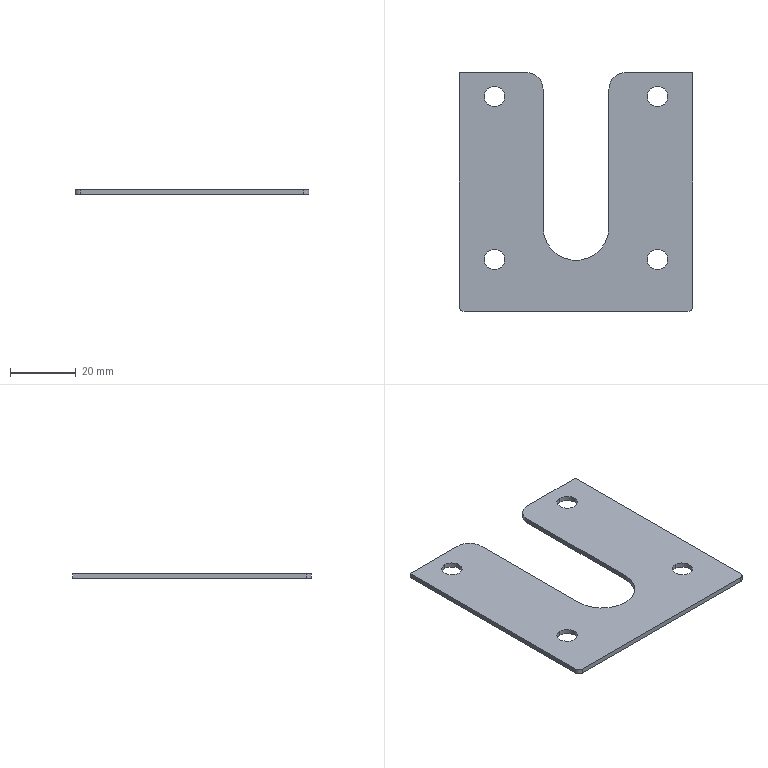Part | NX | features solid 2 | 1 solid | 22 faces | box 71 x 72.5 x 1.5 mm | volume 5877 mm3 | cylinder 13 | plane 9 | commonest cylinder face diameters 6.2 x8 3 x2 10 x2 20 x1
STEP:
#1=CARTESIAN_POINT('',(-1034.749,-1371.151,1295.));
#2=VERTEX_POINT('',#1);
#3=CARTESIAN_POINT('',(-1034.749,-1371.151,1296.5));
#4=VERTEX_POINT('',#3);
#5=CARTESIAN_POINT('',(-1034.749,-1371.151,1395.));
#6=DIRECTION('',(0.,0.,-1.));
#7=VECTOR('',#6,1000.);
#8=LINE('',#5,#7);
#9=EDGE_CURVE('',#2,#4,#8,.F.);
#10=ORIENTED_EDGE('',*,*,#9,.T.);
#11=CARTESIAN_POINT('',(-1034.749,-1377.351,1296.5));
#12=VERTEX_POINT('',#11);
#13=CARTESIAN_POINT('',(-1034.749,-1374.251,1296.5));
#14=DIRECTION('',(0.,0.,1.));
#15=DIRECTION('',(1.,0.,0.));
#16=AXIS2_PLACEMENT_3D('',#13,#14,#15);
#17=CIRCLE('',#16,3.1);
#18=EDGE_CURVE('',#4,#12,#17,.T.);
#19=ORIENTED_EDGE('',*,*,#18,.T.);
#20=CARTESIAN_POINT('',(-1034.749,-1377.351,1295.));
#21=VERTEX_POINT('',#20);
#22=CARTESIAN_POINT('',(-1034.749,-1377.351,1395.));
#23=DIRECTION('',(0.,0.,-1.));
#24=VECTOR('',#23,1000.);
#25=LINE('',#22,#24);
#26=EDGE_CURVE('',#12,#21,#25,.T.);
#27=ORIENTED_EDGE('',*,*,#26,.T.);
#28=CARTESIAN_POINT('',(-1034.749,-1374.251,1295.));
#29=DIRECTION('',(0.,0.,1.));
#30=DIRECTION('',(1.,0.,0.));
#31=AXIS2_PLACEMENT_3D('',#28,#29,#30);
#32=CIRCLE('',#31,3.1);
#33=EDGE_CURVE('',#2,#21,#32,.T.);
#34=ORIENTED_EDGE('',*,*,#33,.F.);
#35=EDGE_LOOP('',(#10,#19,#27,#34));
#36=FACE_BOUND('',#35,.T.);
#37=CARTESIAN_POINT('',(-1034.749,-1374.251,1395.));
#38=DIRECTION('',(0.,0.,-1.));
#39=DIRECTION('',(0.,-1.,0.));
#40=AXIS2_PLACEMENT_3D('',#37,#38,#39);
#41=CYLINDRICAL_SURFACE('',#40,3.1);
#42=ADVANCED_FACE('',(#36),#41,.F.);
#43=CARTESIAN_POINT('',(-1034.749,-1420.649,1296.5));
#44=VERTEX_POINT('',#43);
#45=CARTESIAN_POINT('',(-1034.749,-1420.649,1295.));
#46=VERTEX_POINT('',#45);
#47=CARTESIAN_POINT('',(-1034.749,-1420.649,1395.));
#48=DIRECTION('',(0.,0.,-1.));
#49=VECTOR('',#48,1000.);
#50=LINE('',#47,#49);
#51=EDGE_CURVE('',#44,#46,#50,.T.);
#52=ORIENTED_EDGE('',*,*,#51,.F.);
#53=CARTESIAN_POINT('',(-1034.749,-1426.849,1296.5));
#54=VERTEX_POINT('',#53);
#55=CARTESIAN_POINT('',(-1034.749,-1423.749,1296.5));
#56=DIRECTION('',(0.,0.,1.));
#57=DIRECTION('',(1.,0.,0.));
#58=AXIS2_PLACEMENT_3D('',#55,#56,#57);
#59=CIRCLE('',#58,3.1);
#60=EDGE_CURVE('',#44,#54,#59,.T.);
#61=ORIENTED_EDGE('',*,*,#60,.T.);
#62=CARTESIAN_POINT('',(-1034.749,-1426.849,1295.));
#63=VERTEX_POINT('',#62);
#64=CARTESIAN_POINT('',(-1034.749,-1426.849,1395.));
#65=DIRECTION('',(0.,0.,-1.));
#66=VECTOR('',#65,1000.);
#67=LINE('',#64,#66);
#68=EDGE_CURVE('',#63,#54,#67,.F.);
#69=ORIENTED_EDGE('',*,*,#68,.F.);
#70=CARTESIAN_POINT('',(-1034.749,-1423.749,1295.));
#71=DIRECTION('',(0.,0.,1.));
#72=DIRECTION('',(1.,0.,0.));
#73=AXIS2_PLACEMENT_3D('',#70,#71,#72);
#74=CIRCLE('',#73,3.1);
#75=EDGE_CURVE('',#46,#63,#74,.T.);
#76=ORIENTED_EDGE('',*,*,#75,.F.);
#77=EDGE_LOOP('',(#52,#61,#69,#76));
#78=FACE_BOUND('',#77,.T.);
#79=CARTESIAN_POINT('',(-1034.749,-1423.749,1395.));
#80=DIRECTION('',(0.,0.,-1.));
#81=DIRECTION('',(0.,-1.,0.));
#82=AXIS2_PLACEMENT_3D('',#79,#80,#81);
#83=CYLINDRICAL_SURFACE('',#82,3.1);
#84=ADVANCED_FACE('',(#78),#83,.F.);
#85=CARTESIAN_POINT('',(-985.251,-1420.649,1295.));
#86=VERTEX_POINT('',#85);
#87=CARTESIAN_POINT('',(-985.251,-1420.649,1296.5));
#88=VERTEX_POINT('',#87);
#89=CARTESIAN_POINT('',(-985.251,-1420.649,1395.));
#90=DIRECTION('',(0.,0.,-1.));
#91=VECTOR('',#90,1000.);
#92=LINE('',#89,#91);
#93=EDGE_CURVE('',#86,#88,#92,.F.);
#94=ORIENTED_EDGE('',*,*,#93,.T.);
#95=CARTESIAN_POINT('',(-985.251,-1426.849,1296.5));
#96=VERTEX_POINT('',#95);
#97=CARTESIAN_POINT('',(-985.251,-1423.749,1296.5));
#98=DIRECTION('',(0.,0.,1.));
#99=DIRECTION('',(1.,0.,0.));
#100=AXIS2_PLACEMENT_3D('',#97,#98,#99);
#101=CIRCLE('',#100,3.1);
#102=EDGE_CURVE('',#88,#96,#101,.T.);
#103=ORIENTED_EDGE('',*,*,#102,.T.);
#104=CARTESIAN_POINT('',(-985.251,-1426.849,1295.));
#105=VERTEX_POINT('',#104);
#106=CARTESIAN_POINT('',(-985.251,-1426.849,1395.));
#107=DIRECTION('',(0.,0.,-1.));
#108=VECTOR('',#107,1000.);
#109=LINE('',#106,#108);
#110=EDGE_CURVE('',#96,#105,#109,.T.);
#111=ORIENTED_EDGE('',*,*,#110,.T.);
#112=CARTESIAN_POINT('',(-985.251,-1423.749,1295.));
#113=DIRECTION('',(0.,0.,1.));
#114=DIRECTION('',(1.,0.,0.));
#115=AXIS2_PLACEMENT_3D('',#112,#113,#114);
#116=CIRCLE('',#115,3.1);
#117=EDGE_CURVE('',#86,#105,#116,.T.);
#118=ORIENTED_EDGE('',*,*,#117,.F.);
#119=EDGE_LOOP('',(#94,#103,#111,#118));
#120=FACE_BOUND('',#119,.T.);
#121=CARTESIAN_POINT('',(-985.251,-1423.749,1395.));
#122=DIRECTION('',(0.,0.,-1.));
#123=DIRECTION('',(0.,-1.,0.));
#124=AXIS2_PLACEMENT_3D('',#121,#122,#123);
#125=CYLINDRICAL_SURFACE('',#124,3.1);
#126=ADVANCED_FACE('',(#120),#125,.F.);
#127=CARTESIAN_POINT('',(-985.251,-1371.151,1296.5));
#128=VERTEX_POINT('',#127);
#129=CARTESIAN_POINT('',(-985.251,-1371.151,1295.));
#130=VERTEX_POINT('',#129);
#131=CARTESIAN_POINT('',(-985.251,-1371.151,1395.));
#132=DIRECTION('',(0.,0.,-1.));
#133=VECTOR('',#132,1000.);
#134=LINE('',#131,#133);
#135=EDGE_CURVE('',#128,#130,#134,.T.);
#136=ORIENTED_EDGE('',*,*,#135,.F.);
#137=CARTESIAN_POINT('',(-985.251,-1377.351,1296.5));
#138=VERTEX_POINT('',#137);
#139=CARTESIAN_POINT('',(-985.251,-1374.251,1296.5));
#140=DIRECTION('',(0.,0.,1.));
#141=DIRECTION('',(1.,0.,0.));
#142=AXIS2_PLACEMENT_3D('',#139,#140,#141);
#143=CIRCLE('',#142,3.1);
#144=EDGE_CURVE('',#128,#138,#143,.T.);
#145=ORIENTED_EDGE('',*,*,#144,.T.);
#146=CARTESIAN_POINT('',(-985.251,-1377.351,1295.));
#147=VERTEX_POINT('',#146);
#148=CARTESIAN_POINT('',(-985.251,-1377.351,1395.));
#149=DIRECTION('',(0.,0.,-1.));
#150=VECTOR('',#149,1000.);
#151=LINE('',#148,#150);
#152=EDGE_CURVE('',#147,#138,#151,.F.);
#153=ORIENTED_EDGE('',*,*,#152,.F.);
#154=CARTESIAN_POINT('',(-985.251,-1374.251,1295.));
#155=DIRECTION('',(0.,0.,1.));
#156=DIRECTION('',(1.,0.,0.));
#157=AXIS2_PLACEMENT_3D('',#154,#155,#156);
#158=CIRCLE('',#157,3.1);
#159=EDGE_CURVE('',#130,#147,#158,.T.);
#160=ORIENTED_EDGE('',*,*,#159,.F.);
#161=EDGE_LOOP('',(#136,#145,#153,#160));
#162=FACE_BOUND('',#161,.T.);
#163=CARTESIAN_POINT('',(-985.251,-1374.251,1395.));
#164=DIRECTION('',(0.,0.,-1.));
#165=DIRECTION('',(0.,-1.,0.));
#166=AXIS2_PLACEMENT_3D('',#163,#164,#165);
#167=CYLINDRICAL_SURFACE('',#166,3.1);
#168=ADVANCED_FACE('',(#162),#167,.F.);
#169=CARTESIAN_POINT('',(-995.,-1367.,1296.5));
#170=VERTEX_POINT('',#169);
#171=CARTESIAN_POINT('',(-1000.,-1372.,1296.5));
#172=VERTEX_POINT('',#171);
#173=CARTESIAN_POINT('',(-995.,-1372.,1296.5));
#174=DIRECTION('',(0.,0.,1.));
#175=DIRECTION('',(1.,0.,0.));
#176=AXIS2_PLACEMENT_3D('',#173,#174,#175);
#177=CIRCLE('',#176,5.);
#178=EDGE_CURVE('',#170,#172,#177,.T.);
#179=ORIENTED_EDGE('',*,*,#178,.F.);
#180=CARTESIAN_POINT('',(-995.,-1367.,1295.));
#181=VERTEX_POINT('',#180);
#182=CARTESIAN_POINT('',(-995.,-1367.,1296.5));
#183=DIRECTION('',(0.,0.,1.));
#184=VECTOR('',#183,1000.);
#185=LINE('',#182,#184);
#186=EDGE_CURVE('',#181,#170,#185,.T.);
#187=ORIENTED_EDGE('',*,*,#186,.F.);
#188=CARTESIAN_POINT('',(-1000.,-1372.,1295.));
#189=VERTEX_POINT('',#188);
#190=CARTESIAN_POINT('',(-995.,-1372.,1295.));
#191=DIRECTION('',(0.,0.,-1.));
#192=DIRECTION('',(1.,0.,0.));
#193=AXIS2_PLACEMENT_3D('',#190,#191,#192);
#194=CIRCLE('',#193,5.);
#195=EDGE_CURVE('',#189,#181,#194,.T.);
#196=ORIENTED_EDGE('',*,*,#195,.F.);
#197=CARTESIAN_POINT('',(-1000.,-1372.,1296.5));
#198=DIRECTION('',(0.,0.,-1.));
#199=VECTOR('',#198,1000.);
#200=LINE('',#197,#199);
#201=EDGE_CURVE('',#172,#189,#200,.T.);
#202=ORIENTED_EDGE('',*,*,#201,.F.);
#203=EDGE_LOOP('',(#179,#187,#196,#202));
#204=FACE_BOUND('',#203,.T.);
#205=CARTESIAN_POINT('',(-995.,-1372.,1296.5));
#206=DIRECTION('',(0.,0.,-1.));
#207=DIRECTION('',(-1.,0.,0.));
#208=AXIS2_PLACEMENT_3D('',#205,#206,#207);
#209=CYLINDRICAL_SURFACE('',#208,5.);
#210=ADVANCED_FACE('',(#204),#209,.T.);
#211=CARTESIAN_POINT('',(-1020.,-1372.,1296.5));
#212=VERTEX_POINT('',#211);
#213=CARTESIAN_POINT('',(-1025.,-1367.,1296.5));
#214=VERTEX_POINT('',#213);
#215=CARTESIAN_POINT('',(-1025.,-1372.,1296.5));
#216=DIRECTION('',(0.,0.,1.));
#217=DIRECTION('',(1.,0.,0.));
#218=AXIS2_PLACEMENT_3D('',#215,#216,#217);
#219=CIRCLE('',#218,5.);
#220=EDGE_CURVE('',#212,#214,#219,.T.);
#221=ORIENTED_EDGE('',*,*,#220,.F.);
#222=CARTESIAN_POINT('',(-1020.,-1372.,1295.));
#223=VERTEX_POINT('',#222);
#224=CARTESIAN_POINT('',(-1020.,-1372.,1296.5));
#225=DIRECTION('',(0.,0.,1.));
#226=VECTOR('',#225,1000.);
#227=LINE('',#224,#226);
#228=EDGE_CURVE('',#223,#212,#227,.T.);
#229=ORIENTED_EDGE('',*,*,#228,.F.);
#230=CARTESIAN_POINT('',(-1025.,-1367.,1295.));
#231=VERTEX_POINT('',#230);
#232=CARTESIAN_POINT('',(-1025.,-1372.,1295.));
#233=DIRECTION('',(0.,0.,-1.));
#234=DIRECTION('',(1.,0.,0.));
#235=AXIS2_PLACEMENT_3D('',#232,#233,#234);
#236=CIRCLE('',#235,5.);
#237=EDGE_CURVE('',#231,#223,#236,.T.);
#238=ORIENTED_EDGE('',*,*,#237,.F.);
#239=CARTESIAN_POINT('',(-1025.,-1367.,1296.5));
#240=DIRECTION('',(0.,0.,-1.));
#241=VECTOR('',#240,1000.);
#242=LINE('',#239,#241);
#243=EDGE_CURVE('',#214,#231,#242,.T.);
#244=ORIENTED_EDGE('',*,*,#243,.F.);
#245=EDGE_LOOP('',(#221,#229,#238,#244));
#246=FACE_BOUND('',#245,.T.);
#247=CARTESIAN_POINT('',(-1025.,-1372.,1296.5));
#248=DIRECTION('',(0.,0.,-1.));
#249=DIRECTION('',(-1.,0.,0.));
#250=AXIS2_PLACEMENT_3D('',#247,#248,#249);
#251=CYLINDRICAL_SURFACE('',#250,5.);
#252=ADVANCED_FACE('',(#246),#251,.T.);
#253=CARTESIAN_POINT('',(-985.251,-1374.251,1295.));
#254=DIRECTION('',(0.,0.,1.));
#255=DIRECTION('',(1.,0.,0.));
#256=AXIS2_PLACEMENT_3D('',#253,#254,#255);
#257=CIRCLE('',#256,3.1);
#258=EDGE_CURVE('',#147,#130,#257,.T.);
#259=ORIENTED_EDGE('',*,*,#258,.T.);
#260=ORIENTED_EDGE('',*,*,#159,.T.);
#261=EDGE_LOOP('',(#259,#260));
#262=FACE_BOUND('',#261,.T.);
#263=CARTESIAN_POINT('',(-985.251,-1423.749,1295.));
#264=DIRECTION('',(0.,0.,1.));
#265=DIRECTION('',(1.,0.,0.));
#266=AXIS2_PLACEMENT_3D('',#263,#264,#265);
#267=CIRCLE('',#266,3.1);
#268=EDGE_CURVE('',#105,#86,#267,.T.);
#269=ORIENTED_EDGE('',*,*,#268,.T.);
#270=ORIENTED_EDGE('',*,*,#117,.T.);
#271=EDGE_LOOP('',(#269,#270));
#272=FACE_BOUND('',#271,.T.);
#273=CARTESIAN_POINT('',(-1034.749,-1423.749,1295.));
#274=DIRECTION('',(0.,0.,1.));
#275=DIRECTION('',(1.,0.,0.));
#276=AXIS2_PLACEMENT_3D('',#273,#274,#275);
#277=CIRCLE('',#276,3.1);
#278=EDGE_CURVE('',#63,#46,#277,.T.);
#279=ORIENTED_EDGE('',*,*,#278,.T.);
#280=ORIENTED_EDGE('',*,*,#75,.T.);
#281=EDGE_LOOP('',(#279,#280));
#282=FACE_BOUND('',#281,.T.);
#283=CARTESIAN_POINT('',(-1034.749,-1374.251,1295.));
#284=DIRECTION('',(0.,0.,1.));
#285=DIRECTION('',(1.,0.,0.));
#286=AXIS2_PLACEMENT_3D('',#283,#284,#285);
#287=CIRCLE('',#286,3.1);
#288=EDGE_CURVE('',#21,#2,#287,.T.);
#289=ORIENTED_EDGE('',*,*,#288,.T.);
#290=ORIENTED_EDGE('',*,*,#33,.T.);
#291=EDGE_LOOP('',(#289,#290));
#292=FACE_BOUND('',#291,.T.);
#293=CARTESIAN_POINT('',(-1045.5,-1367.,1295.));
#294=VERTEX_POINT('',#293);
#295=CARTESIAN_POINT('',(-1045.5,-1367.,1295.));
#296=DIRECTION('',(-1.,0.,0.));
#297=VECTOR('',#296,1000.);
#298=LINE('',#295,#297);
#299=EDGE_CURVE('',#231,#294,#298,.T.);
#300=ORIENTED_EDGE('',*,*,#299,.F.);
#301=ORIENTED_EDGE('',*,*,#237,.T.);
#302=CARTESIAN_POINT('',(-1020.,-1414.,1295.));
#303=VERTEX_POINT('',#302);
#304=CARTESIAN_POINT('',(-1020.,-1414.,1295.));
#305=DIRECTION('',(0.,1.,0.));
#306=VECTOR('',#305,1000.);
#307=LINE('',#304,#306);
#308=EDGE_CURVE('',#303,#223,#307,.T.);
#309=ORIENTED_EDGE('',*,*,#308,.F.);
#310=CARTESIAN_POINT('',(-1000.,-1414.,1295.));
#311=VERTEX_POINT('',#310);
#312=CARTESIAN_POINT('',(-1010.,-1414.,1295.));
#313=DIRECTION('',(0.,0.,-1.));
#314=DIRECTION('',(1.,0.,0.));
#315=AXIS2_PLACEMENT_3D('',#312,#313,#314);
#316=CIRCLE('',#315,10.);
#317=EDGE_CURVE('',#311,#303,#316,.T.);
#318=ORIENTED_EDGE('',*,*,#317,.F.);
#319=CARTESIAN_POINT('',(-1000.,-1414.,1295.));
#320=DIRECTION('',(0.,-1.,0.));
#321=VECTOR('',#320,1000.);
#322=LINE('',#319,#321);
#323=EDGE_CURVE('',#189,#311,#322,.T.);
#324=ORIENTED_EDGE('',*,*,#323,.F.);
#325=ORIENTED_EDGE('',*,*,#195,.T.);
#326=CARTESIAN_POINT('',(-974.5,-1367.,1295.));
#327=VERTEX_POINT('',#326);
#328=CARTESIAN_POINT('',(-1000.,-1367.,1295.));
#329=DIRECTION('',(-1.,0.,0.));
#330=VECTOR('',#329,1000.);
#331=LINE('',#328,#330);
#332=EDGE_CURVE('',#327,#181,#331,.T.);
#333=ORIENTED_EDGE('',*,*,#332,.F.);
#334=CARTESIAN_POINT('',(-974.5,-1438.,1295.));
#335=VERTEX_POINT('',#334);
#336=CARTESIAN_POINT('',(-974.5,-1438.,1295.));
#337=DIRECTION('',(0.,1.,0.));
#338=VECTOR('',#337,1000.);
#339=LINE('',#336,#338);
#340=EDGE_CURVE('',#335,#327,#339,.T.);
#341=ORIENTED_EDGE('',*,*,#340,.F.);
#342=CARTESIAN_POINT('',(-976.,-1439.5,1295.));
#343=VERTEX_POINT('',#342);
#344=CARTESIAN_POINT('',(-976.,-1438.,1295.));
#345=DIRECTION('',(0.,0.,1.));
#346=DIRECTION('',(-1.,0.,0.));
#347=AXIS2_PLACEMENT_3D('',#344,#345,#346);
#348=CIRCLE('',#347,1.5);
#349=EDGE_CURVE('',#343,#335,#348,.T.);
#350=ORIENTED_EDGE('',*,*,#349,.F.);
#351=CARTESIAN_POINT('',(-1044.,-1439.5,1295.));
#352=VERTEX_POINT('',#351);
#353=CARTESIAN_POINT('',(-1044.,-1439.5,1295.));
#354=DIRECTION('',(1.,0.,0.));
#355=VECTOR('',#354,1000.);
#356=LINE('',#353,#355);
#357=EDGE_CURVE('',#352,#343,#356,.T.);
#358=ORIENTED_EDGE('',*,*,#357,.F.);
#359=CARTESIAN_POINT('',(-1045.5,-1438.,1295.));
#360=VERTEX_POINT('',#359);
#361=CARTESIAN_POINT('',(-1044.,-1438.,1295.));
#362=DIRECTION('',(0.,0.,1.));
#363=DIRECTION('',(1.,0.,0.));
#364=AXIS2_PLACEMENT_3D('',#361,#362,#363);
#365=CIRCLE('',#364,1.5);
#366=EDGE_CURVE('',#360,#352,#365,.T.);
#367=ORIENTED_EDGE('',*,*,#366,.F.);
#368=CARTESIAN_POINT('',(-1045.5,-1367.,1295.));
#369=DIRECTION('',(0.,-1.,0.));
#370=VECTOR('',#369,1000.);
#371=LINE('',#368,#370);
#372=EDGE_CURVE('',#294,#360,#371,.T.);
#373=ORIENTED_EDGE('',*,*,#372,.F.);
#374=EDGE_LOOP('',(#300,#301,#309,#318,#324,#325,#333,#341,#350,#358,#367,#373));
#375=FACE_BOUND('',#374,.T.);
#376=CARTESIAN_POINT('',(-1044.,-1438.,1295.));
#377=DIRECTION('',(0.,0.,1.));
#378=DIRECTION('',(1.,0.,0.));
#379=AXIS2_PLACEMENT_3D('',#376,#377,#378);
#380=PLANE('',#379);
#381=ADVANCED_FACE('',(#262,#272,#282,#292,#375),#380,.F.);
#382=CARTESIAN_POINT('',(-985.251,-1374.251,1296.5));
#383=DIRECTION('',(0.,0.,1.));
#384=DIRECTION('',(1.,0.,0.));
#385=AXIS2_PLACEMENT_3D('',#382,#383,#384);
#386=CIRCLE('',#385,3.1);
#387=EDGE_CURVE('',#138,#128,#386,.T.);
#388=ORIENTED_EDGE('',*,*,#387,.F.);
#389=ORIENTED_EDGE('',*,*,#144,.F.);
#390=EDGE_LOOP('',(#388,#389));
#391=FACE_BOUND('',#390,.T.);
#392=CARTESIAN_POINT('',(-985.251,-1423.749,1296.5));
#393=DIRECTION('',(0.,0.,1.));
#394=DIRECTION('',(1.,0.,0.));
#395=AXIS2_PLACEMENT_3D('',#392,#393,#394);
#396=CIRCLE('',#395,3.1);
#397=EDGE_CURVE('',#96,#88,#396,.T.);
#398=ORIENTED_EDGE('',*,*,#397,.F.);
#399=ORIENTED_EDGE('',*,*,#102,.F.);
#400=EDGE_LOOP('',(#398,#399));
#401=FACE_BOUND('',#400,.T.);
#402=CARTESIAN_POINT('',(-1034.749,-1423.749,1296.5));
#403=DIRECTION('',(0.,0.,1.));
#404=DIRECTION('',(1.,0.,0.));
#405=AXIS2_PLACEMENT_3D('',#402,#403,#404);
#406=CIRCLE('',#405,3.1);
#407=EDGE_CURVE('',#54,#44,#406,.T.);
#408=ORIENTED_EDGE('',*,*,#407,.F.);
#409=ORIENTED_EDGE('',*,*,#60,.F.);
#410=EDGE_LOOP('',(#408,#409));
#411=FACE_BOUND('',#410,.T.);
#412=CARTESIAN_POINT('',(-1034.749,-1374.251,1296.5));
#413=DIRECTION('',(0.,0.,1.));
#414=DIRECTION('',(1.,0.,0.));
#415=AXIS2_PLACEMENT_3D('',#412,#413,#414);
#416=CIRCLE('',#415,3.1);
#417=EDGE_CURVE('',#12,#4,#416,.T.);
#418=ORIENTED_EDGE('',*,*,#417,.F.);
#419=ORIENTED_EDGE('',*,*,#18,.F.);
#420=EDGE_LOOP('',(#418,#419));
#421=FACE_BOUND('',#420,.T.);
#422=CARTESIAN_POINT('',(-1020.,-1414.,1296.5));
#423=VERTEX_POINT('',#422);
#424=CARTESIAN_POINT('',(-1020.,-1414.,1296.5));
#425=DIRECTION('',(0.,1.,0.));
#426=VECTOR('',#425,1000.);
#427=LINE('',#424,#426);
#428=EDGE_CURVE('',#423,#212,#427,.T.);
#429=ORIENTED_EDGE('',*,*,#428,.T.);
#430=ORIENTED_EDGE('',*,*,#220,.T.);
#431=CARTESIAN_POINT('',(-1045.5,-1367.,1296.5));
#432=VERTEX_POINT('',#431);
#433=CARTESIAN_POINT('',(-1045.5,-1367.,1296.5));
#434=DIRECTION('',(-1.,0.,0.));
#435=VECTOR('',#434,1000.);
#436=LINE('',#433,#435);
#437=EDGE_CURVE('',#214,#432,#436,.T.);
#438=ORIENTED_EDGE('',*,*,#437,.T.);
#439=CARTESIAN_POINT('',(-1045.5,-1438.,1296.5));
#440=VERTEX_POINT('',#439);
#441=CARTESIAN_POINT('',(-1045.5,-1367.,1296.5));
#442=DIRECTION('',(0.,-1.,0.));
#443=VECTOR('',#442,1000.);
#444=LINE('',#441,#443);
#445=EDGE_CURVE('',#432,#440,#444,.T.);
#446=ORIENTED_EDGE('',*,*,#445,.T.);
#447=CARTESIAN_POINT('',(-1044.,-1439.5,1296.5));
#448=VERTEX_POINT('',#447);
#449=CARTESIAN_POINT('',(-1044.,-1438.,1296.5));
#450=DIRECTION('',(0.,0.,1.));
#451=DIRECTION('',(1.,0.,0.));
#452=AXIS2_PLACEMENT_3D('',#449,#450,#451);
#453=CIRCLE('',#452,1.5);
#454=EDGE_CURVE('',#440,#448,#453,.T.);
#455=ORIENTED_EDGE('',*,*,#454,.T.);
#456=CARTESIAN_POINT('',(-976.,-1439.5,1296.5));
#457=VERTEX_POINT('',#456);
#458=CARTESIAN_POINT('',(-1044.,-1439.5,1296.5));
#459=DIRECTION('',(1.,0.,0.));
#460=VECTOR('',#459,1000.);
#461=LINE('',#458,#460);
#462=EDGE_CURVE('',#448,#457,#461,.T.);
#463=ORIENTED_EDGE('',*,*,#462,.T.);
#464=CARTESIAN_POINT('',(-974.5,-1438.,1296.5));
#465=VERTEX_POINT('',#464);
#466=CARTESIAN_POINT('',(-976.,-1438.,1296.5));
#467=DIRECTION('',(0.,0.,1.));
#468=DIRECTION('',(-1.,0.,0.));
#469=AXIS2_PLACEMENT_3D('',#466,#467,#468);
#470=CIRCLE('',#469,1.5);
#471=EDGE_CURVE('',#457,#465,#470,.T.);
#472=ORIENTED_EDGE('',*,*,#471,.T.);
#473=CARTESIAN_POINT('',(-974.5,-1367.,1296.5));
#474=VERTEX_POINT('',#473);
#475=CARTESIAN_POINT('',(-974.5,-1438.,1296.5));
#476=DIRECTION('',(0.,1.,0.));
#477=VECTOR('',#476,1000.);
#478=LINE('',#475,#477);
#479=EDGE_CURVE('',#465,#474,#478,.T.);
#480=ORIENTED_EDGE('',*,*,#479,.T.);
#481=CARTESIAN_POINT('',(-1000.,-1367.,1296.5));
#482=DIRECTION('',(-1.,0.,0.));
#483=VECTOR('',#482,1000.);
#484=LINE('',#481,#483);
#485=EDGE_CURVE('',#474,#170,#484,.T.);
#486=ORIENTED_EDGE('',*,*,#485,.T.);
#487=ORIENTED_EDGE('',*,*,#178,.T.);
#488=CARTESIAN_POINT('',(-1000.,-1414.,1296.5));
#489=VERTEX_POINT('',#488);
#490=CARTESIAN_POINT('',(-1000.,-1414.,1296.5));
#491=DIRECTION('',(0.,-1.,0.));
#492=VECTOR('',#491,1000.);
#493=LINE('',#490,#492);
#494=EDGE_CURVE('',#172,#489,#493,.T.);
#495=ORIENTED_EDGE('',*,*,#494,.T.);
#496=CARTESIAN_POINT('',(-1010.,-1414.,1296.5));
#497=DIRECTION('',(0.,0.,-1.));
#498=DIRECTION('',(1.,0.,0.));
#499=AXIS2_PLACEMENT_3D('',#496,#497,#498);
#500=CIRCLE('',#499,10.);
#501=EDGE_CURVE('',#489,#423,#500,.T.);
#502=ORIENTED_EDGE('',*,*,#501,.T.);
#503=EDGE_LOOP('',(#429,#430,#438,#446,#455,#463,#472,#480,#486,#487,#495,#502));
#504=FACE_BOUND('',#503,.T.);
#505=CARTESIAN_POINT('',(-1044.,-1438.,1296.5));
#506=DIRECTION('',(0.,0.,1.));
#507=DIRECTION('',(1.,0.,0.));
#508=AXIS2_PLACEMENT_3D('',#505,#506,#507);
#509=PLANE('',#508);
#510=ADVANCED_FACE('',(#391,#401,#411,#421,#504),#509,.T.);
#511=ORIENTED_EDGE('',*,*,#372,.T.);
#512=CARTESIAN_POINT('',(-1045.5,-1438.,1296.5));
#513=DIRECTION('',(0.,0.,-1.));
#514=VECTOR('',#513,1000.);
#515=LINE('',#512,#514);
#516=EDGE_CURVE('',#440,#360,#515,.T.);
#517=ORIENTED_EDGE('',*,*,#516,.F.);
#518=ORIENTED_EDGE('',*,*,#445,.F.);
#519=CARTESIAN_POINT('',(-1045.5,-1367.,1296.5));
#520=DIRECTION('',(0.,0.,-1.));
#521=VECTOR('',#520,1000.);
#522=LINE('',#519,#521);
#523=EDGE_CURVE('',#432,#294,#522,.T.);
#524=ORIENTED_EDGE('',*,*,#523,.T.);
#525=EDGE_LOOP('',(#511,#517,#518,#524));
#526=FACE_BOUND('',#525,.T.);
#527=CARTESIAN_POINT('',(-1045.5,-1367.,1296.5));
#528=DIRECTION('',(1.,0.,0.));
#529=DIRECTION('',(0.,-1.,0.));
#530=AXIS2_PLACEMENT_3D('',#527,#528,#529);
#531=PLANE('',#530);
#532=ADVANCED_FACE('',(#526),#531,.F.);
#533=ORIENTED_EDGE('',*,*,#437,.F.);
#534=ORIENTED_EDGE('',*,*,#243,.T.);
#535=ORIENTED_EDGE('',*,*,#299,.T.);
#536=ORIENTED_EDGE('',*,*,#523,.F.);
#537=EDGE_LOOP('',(#533,#534,#535,#536));
#538=FACE_BOUND('',#537,.T.);
#539=CARTESIAN_POINT('',(-1045.5,-1367.,1296.5));
#540=DIRECTION('',(0.,-1.,0.));
#541=DIRECTION('',(0.,0.,-1.));
#542=AXIS2_PLACEMENT_3D('',#539,#540,#541);
#543=PLANE('',#542);
#544=ADVANCED_FACE('',(#538),#543,.F.);
#545=ORIENTED_EDGE('',*,*,#308,.T.);
#546=ORIENTED_EDGE('',*,*,#228,.T.);
#547=ORIENTED_EDGE('',*,*,#428,.F.);
#548=CARTESIAN_POINT('',(-1020.,-1414.,1296.5));
#549=DIRECTION('',(0.,0.,-1.));
#550=VECTOR('',#549,1000.);
#551=LINE('',#548,#550);
#552=EDGE_CURVE('',#423,#303,#551,.T.);
#553=ORIENTED_EDGE('',*,*,#552,.T.);
#554=EDGE_LOOP('',(#545,#546,#547,#553));
#555=FACE_BOUND('',#554,.T.);
#556=CARTESIAN_POINT('',(-1020.,-1414.,1296.5));
#557=DIRECTION('',(-1.,0.,0.));
#558=DIRECTION('',(0.,0.,1.));
#559=AXIS2_PLACEMENT_3D('',#556,#557,#558);
#560=PLANE('',#559);
#561=ADVANCED_FACE('',(#555),#560,.F.);
#562=ORIENTED_EDGE('',*,*,#317,.T.);
#563=ORIENTED_EDGE('',*,*,#552,.F.);
#564=ORIENTED_EDGE('',*,*,#501,.F.);
#565=CARTESIAN_POINT('',(-1000.,-1414.,1296.5));
#566=DIRECTION('',(0.,0.,-1.));
#567=VECTOR('',#566,1000.);
#568=LINE('',#565,#567);
#569=EDGE_CURVE('',#489,#311,#568,.T.);
#570=ORIENTED_EDGE('',*,*,#569,.T.);
#571=EDGE_LOOP('',(#562,#563,#564,#570));
#572=FACE_BOUND('',#571,.T.);
#573=CARTESIAN_POINT('',(-1010.,-1414.,1296.5));
#574=DIRECTION('',(0.,0.,-1.));
#575=DIRECTION('',(-1.,0.,0.));
#576=AXIS2_PLACEMENT_3D('',#573,#574,#575);
#577=CYLINDRICAL_SURFACE('',#576,10.);
#578=ADVANCED_FACE('',(#572),#577,.F.);
#579=ORIENTED_EDGE('',*,*,#494,.F.);
#580=ORIENTED_EDGE('',*,*,#201,.T.);
#581=ORIENTED_EDGE('',*,*,#323,.T.);
#582=ORIENTED_EDGE('',*,*,#569,.F.);
#583=EDGE_LOOP('',(#579,#580,#581,#582));
#584=FACE_BOUND('',#583,.T.);
#585=CARTESIAN_POINT('',(-1000.,-1414.,1296.5));
#586=DIRECTION('',(1.,0.,0.));
#587=DIRECTION('',(0.,-1.,0.));
#588=AXIS2_PLACEMENT_3D('',#585,#586,#587);
#589=PLANE('',#588);
#590=ADVANCED_FACE('',(#584),#589,.F.);
#591=ORIENTED_EDGE('',*,*,#332,.T.);
#592=ORIENTED_EDGE('',*,*,#186,.T.);
#593=ORIENTED_EDGE('',*,*,#485,.F.);
#594=CARTESIAN_POINT('',(-974.5,-1367.,1296.5));
#595=DIRECTION('',(0.,0.,-1.));
#596=VECTOR('',#595,1000.);
#597=LINE('',#594,#596);
#598=EDGE_CURVE('',#474,#327,#597,.T.);
#599=ORIENTED_EDGE('',*,*,#598,.T.);
#600=EDGE_LOOP('',(#591,#592,#593,#599));
#601=FACE_BOUND('',#600,.T.);
#602=CARTESIAN_POINT('',(-1000.,-1367.,1296.5));
#603=DIRECTION('',(0.,-1.,0.));
#604=DIRECTION('',(0.,0.,-1.));
#605=AXIS2_PLACEMENT_3D('',#602,#603,#604);
#606=PLANE('',#605);
#607=ADVANCED_FACE('',(#601),#606,.F.);
#608=ORIENTED_EDGE('',*,*,#340,.T.);
#609=ORIENTED_EDGE('',*,*,#598,.F.);
#610=ORIENTED_EDGE('',*,*,#479,.F.);
#611=CARTESIAN_POINT('',(-974.5,-1438.,1296.5));
#612=DIRECTION('',(0.,0.,-1.));
#613=VECTOR('',#612,1000.);
#614=LINE('',#611,#613);
#615=EDGE_CURVE('',#465,#335,#614,.T.);
#616=ORIENTED_EDGE('',*,*,#615,.T.);
#617=EDGE_LOOP('',(#608,#609,#610,#616));
#618=FACE_BOUND('',#617,.T.);
#619=CARTESIAN_POINT('',(-974.5,-1438.,1296.5));
#620=DIRECTION('',(-1.,0.,0.));
#621=DIRECTION('',(0.,0.,1.));
#622=AXIS2_PLACEMENT_3D('',#619,#620,#621);
#623=PLANE('',#622);
#624=ADVANCED_FACE('',(#618),#623,.F.);
#625=ORIENTED_EDGE('',*,*,#349,.T.);
#626=ORIENTED_EDGE('',*,*,#615,.F.);
#627=ORIENTED_EDGE('',*,*,#471,.F.);
#628=CARTESIAN_POINT('',(-976.,-1439.5,1296.5));
#629=DIRECTION('',(0.,0.,-1.));
#630=VECTOR('',#629,1000.);
#631=LINE('',#628,#630);
#632=EDGE_CURVE('',#457,#343,#631,.T.);
#633=ORIENTED_EDGE('',*,*,#632,.T.);
#634=EDGE_LOOP('',(#625,#626,#627,#633));
#635=FACE_BOUND('',#634,.T.);
#636=CARTESIAN_POINT('',(-976.,-1438.,1296.5));
#637=DIRECTION('',(0.,0.,-1.));
#638=DIRECTION('',(-1.,0.,0.));
#639=AXIS2_PLACEMENT_3D('',#636,#637,#638);
#640=CYLINDRICAL_SURFACE('',#639,1.5);
#641=ADVANCED_FACE('',(#635),#640,.T.);
#642=ORIENTED_EDGE('',*,*,#357,.T.);
#643=ORIENTED_EDGE('',*,*,#632,.F.);
#644=ORIENTED_EDGE('',*,*,#462,.F.);
#645=CARTESIAN_POINT('',(-1044.,-1439.5,1296.5));
#646=DIRECTION('',(0.,0.,-1.));
#647=VECTOR('',#646,1000.);
#648=LINE('',#645,#647);
#649=EDGE_CURVE('',#448,#352,#648,.T.);
#650=ORIENTED_EDGE('',*,*,#649,.T.);
#651=EDGE_LOOP('',(#642,#643,#644,#650));
#652=FACE_BOUND('',#651,.T.);
#653=CARTESIAN_POINT('',(-1044.,-1439.5,1296.5));
#654=DIRECTION('',(0.,1.,0.));
#655=DIRECTION('',(1.,0.,0.));
#656=AXIS2_PLACEMENT_3D('',#653,#654,#655);
#657=PLANE('',#656);
#658=ADVANCED_FACE('',(#652),#657,.F.);
#659=ORIENTED_EDGE('',*,*,#366,.T.);
#660=ORIENTED_EDGE('',*,*,#649,.F.);
#661=ORIENTED_EDGE('',*,*,#454,.F.);
#662=ORIENTED_EDGE('',*,*,#516,.T.);
#663=EDGE_LOOP('',(#659,#660,#661,#662));
#664=FACE_BOUND('',#663,.T.);
#665=CARTESIAN_POINT('',(-1044.,-1438.,1296.5));
#666=DIRECTION('',(0.,0.,-1.));
#667=DIRECTION('',(-1.,0.,0.));
#668=AXIS2_PLACEMENT_3D('',#665,#666,#667);
#669=CYLINDRICAL_SURFACE('',#668,1.5);
#670=ADVANCED_FACE('',(#664),#669,.T.);
#671=ORIENTED_EDGE('',*,*,#387,.T.);
#672=ORIENTED_EDGE('',*,*,#135,.T.);
#673=ORIENTED_EDGE('',*,*,#258,.F.);
#674=ORIENTED_EDGE('',*,*,#152,.T.);
#675=EDGE_LOOP('',(#671,#672,#673,#674));
#676=FACE_BOUND('',#675,.T.);
#677=CARTESIAN_POINT('',(-985.251,-1374.251,1395.));
#678=DIRECTION('',(0.,0.,-1.));
#679=DIRECTION('',(0.,-1.,0.));
#680=AXIS2_PLACEMENT_3D('',#677,#678,#679);
#681=CYLINDRICAL_SURFACE('',#680,3.1);
#682=ADVANCED_FACE('',(#676),#681,.F.);
#683=ORIENTED_EDGE('',*,*,#397,.T.);
#684=ORIENTED_EDGE('',*,*,#93,.F.);
#685=ORIENTED_EDGE('',*,*,#268,.F.);
#686=ORIENTED_EDGE('',*,*,#110,.F.);
#687=EDGE_LOOP('',(#683,#684,#685,#686));
#688=FACE_BOUND('',#687,.T.);
#689=CARTESIAN_POINT('',(-985.251,-1423.749,1395.));
#690=DIRECTION('',(0.,0.,-1.));
#691=DIRECTION('',(0.,-1.,0.));
#692=AXIS2_PLACEMENT_3D('',#689,#690,#691);
#693=CYLINDRICAL_SURFACE('',#692,3.1);
#694=ADVANCED_FACE('',(#688),#693,.F.);
#695=ORIENTED_EDGE('',*,*,#407,.T.);
#696=ORIENTED_EDGE('',*,*,#51,.T.);
#697=ORIENTED_EDGE('',*,*,#278,.F.);
#698=ORIENTED_EDGE('',*,*,#68,.T.);
#699=EDGE_LOOP('',(#695,#696,#697,#698));
#700=FACE_BOUND('',#699,.T.);
#701=CARTESIAN_POINT('',(-1034.749,-1423.749,1395.));
#702=DIRECTION('',(0.,0.,-1.));
#703=DIRECTION('',(0.,-1.,0.));
#704=AXIS2_PLACEMENT_3D('',#701,#702,#703);
#705=CYLINDRICAL_SURFACE('',#704,3.1);
#706=ADVANCED_FACE('',(#700),#705,.F.);
#707=ORIENTED_EDGE('',*,*,#417,.T.);
#708=ORIENTED_EDGE('',*,*,#9,.F.);
#709=ORIENTED_EDGE('',*,*,#288,.F.);
#710=ORIENTED_EDGE('',*,*,#26,.F.);
#711=EDGE_LOOP('',(#707,#708,#709,#710));
#712=FACE_BOUND('',#711,.T.);
#713=CARTESIAN_POINT('',(-1034.749,-1374.251,1395.));
#714=DIRECTION('',(0.,0.,-1.));
#715=DIRECTION('',(0.,-1.,0.));
#716=AXIS2_PLACEMENT_3D('',#713,#714,#715);
#717=CYLINDRICAL_SURFACE('',#716,3.1);
#718=ADVANCED_FACE('',(#712),#717,.F.);
#719=CLOSED_SHELL('',(#42,#84,#126,#168,#210,#252,#381,#510,#532,#544,#561,#578,#590,#607,#624,#641,#658,#670,#682,#694,#706,#718));
#720=MANIFOLD_SOLID_BREP('',#719);
#721=(LENGTH_UNIT()NAMED_UNIT(*)SI_UNIT(.MILLI.,.METRE.));
#722=UNCERTAINTY_MEASURE_WITH_UNIT(LENGTH_MEASURE(0.00001),#721,'','');
#723=(NAMED_UNIT(*)PLANE_ANGLE_UNIT()SI_UNIT($,.RADIAN.));
#724=(NAMED_UNIT(*)SI_UNIT($,.STERADIAN.)SOLID_ANGLE_UNIT());
#725=(GEOMETRIC_REPRESENTATION_CONTEXT(3)GLOBAL_UNCERTAINTY_ASSIGNED_CONTEXT((#722))GLOBAL_UNIT_ASSIGNED_CONTEXT((#721,#723,#724))REPRESENTATION_CONTEXT('',''));
#726=ADVANCED_BREP_SHAPE_REPRESENTATION('',(#720),#725);